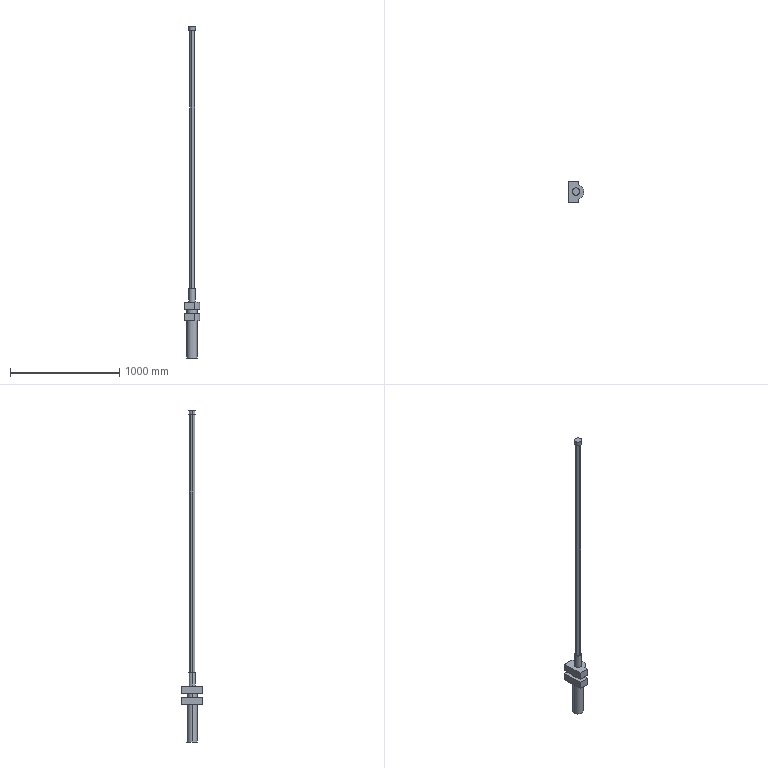Part | SolidWorks | features ICE 4, Extrusion 1, Revolution 1 | 1 solid | 34 faces | box 145 x 200 x 3045 mm | volume 9881039 mm3 | plane 24 | cylinder 8 | cone 2 | commonest cylinder face diameters 92.4 x4 60 x2 145 x2
STEP:
#1=CARTESIAN_POINT('',(46.2,0.,340.));
#2=VERTEX_POINT('',#1);
#3=CARTESIAN_POINT('',(-46.2,0.,340.));
#4=VERTEX_POINT('',#3);
#5=CARTESIAN_POINT('',(0.,0.,340.));
#6=DIRECTION('',(0.,0.,1.));
#7=DIRECTION('',(1.,0.,0.));
#8=AXIS2_PLACEMENT_3D('',#5,#6,#7);
#9=CIRCLE('',#8,46.2);
#10=EDGE_CURVE('',#2,#4,#9,.T.);
#11=ORIENTED_EDGE('',*,*,#10,.F.);
#12=CARTESIAN_POINT('',(46.2,0.,0.));
#13=VERTEX_POINT('',#12);
#14=CARTESIAN_POINT('',(46.2,0.,445.));
#15=DIRECTION('',(0.,0.,-1.));
#16=VECTOR('',#15,1000.);
#17=LINE('',#14,#16);
#18=EDGE_CURVE('',#2,#13,#17,.T.);
#19=ORIENTED_EDGE('',*,*,#18,.T.);
#20=CARTESIAN_POINT('',(-46.2,0.,0.));
#21=VERTEX_POINT('',#20);
#22=CARTESIAN_POINT('',(0.,0.,0.));
#23=DIRECTION('',(0.,0.,1.));
#24=DIRECTION('',(1.,0.,0.));
#25=AXIS2_PLACEMENT_3D('',#22,#23,#24);
#26=CIRCLE('',#25,46.2);
#27=EDGE_CURVE('',#13,#21,#26,.T.);
#28=ORIENTED_EDGE('',*,*,#27,.T.);
#29=CARTESIAN_POINT('',(-46.2,0.,445.));
#30=DIRECTION('',(0.,0.,-1.));
#31=VECTOR('',#30,1000.);
#32=LINE('',#29,#31);
#33=EDGE_CURVE('',#4,#21,#32,.T.);
#34=ORIENTED_EDGE('',*,*,#33,.F.);
#35=EDGE_LOOP('',(#11,#19,#28,#34));
#36=FACE_OUTER_BOUND('',#35,.T.);
#37=CARTESIAN_POINT('',(0.,0.,445.));
#38=DIRECTION('',(0.,0.,-1.));
#39=DIRECTION('',(-1.,0.,0.));
#40=AXIS2_PLACEMENT_3D('',#37,#38,#39);
#41=CYLINDRICAL_SURFACE('',#40,46.2);
#42=ADVANCED_FACE('',(#36),#41,.T.);
#43=CARTESIAN_POINT('',(46.2,0.,445.));
#44=VERTEX_POINT('',#43);
#45=CARTESIAN_POINT('',(-46.2,0.,445.));
#46=VERTEX_POINT('',#45);
#47=CARTESIAN_POINT('',(0.,0.,445.));
#48=DIRECTION('',(0.,0.,1.));
#49=DIRECTION('',(1.,0.,0.));
#50=AXIS2_PLACEMENT_3D('',#47,#48,#49);
#51=CIRCLE('',#50,46.2);
#52=EDGE_CURVE('',#44,#46,#51,.T.);
#53=ORIENTED_EDGE('',*,*,#52,.F.);
#54=CARTESIAN_POINT('',(46.2,0.,408.));
#55=VERTEX_POINT('',#54);
#56=CARTESIAN_POINT('',(46.2,0.,445.));
#57=DIRECTION('',(0.,0.,-1.));
#58=VECTOR('',#57,1000.);
#59=LINE('',#56,#58);
#60=EDGE_CURVE('',#44,#55,#59,.T.);
#61=ORIENTED_EDGE('',*,*,#60,.T.);
#62=CARTESIAN_POINT('',(-46.2,0.,408.));
#63=VERTEX_POINT('',#62);
#64=CARTESIAN_POINT('',(0.,0.,408.));
#65=DIRECTION('',(0.,0.,1.));
#66=DIRECTION('',(1.,0.,0.));
#67=AXIS2_PLACEMENT_3D('',#64,#65,#66);
#68=CIRCLE('',#67,46.2);
#69=EDGE_CURVE('',#55,#63,#68,.T.);
#70=ORIENTED_EDGE('',*,*,#69,.T.);
#71=CARTESIAN_POINT('',(-46.2,0.,445.));
#72=DIRECTION('',(0.,0.,-1.));
#73=VECTOR('',#72,1000.);
#74=LINE('',#71,#73);
#75=EDGE_CURVE('',#46,#63,#74,.T.);
#76=ORIENTED_EDGE('',*,*,#75,.F.);
#77=EDGE_LOOP('',(#53,#61,#70,#76));
#78=FACE_OUTER_BOUND('',#77,.T.);
#79=CARTESIAN_POINT('',(0.,0.,445.));
#80=DIRECTION('',(0.,0.,-1.));
#81=DIRECTION('',(-1.,0.,0.));
#82=AXIS2_PLACEMENT_3D('',#79,#80,#81);
#83=CYLINDRICAL_SURFACE('',#82,46.2);
#84=ADVANCED_FACE('',(#78),#83,.T.);
#85=CARTESIAN_POINT('',(-29.4,0.,3000.));
#86=VERTEX_POINT('',#85);
#87=CARTESIAN_POINT('',(29.4,0.,3000.));
#88=VERTEX_POINT('',#87);
#89=CARTESIAN_POINT('',(0.,0.,3000.));
#90=DIRECTION('',(0.,0.,-1.));
#91=DIRECTION('',(-1.,0.,0.));
#92=AXIS2_PLACEMENT_3D('',#89,#90,#91);
#93=CIRCLE('',#92,29.4);
#94=EDGE_CURVE('',#86,#88,#93,.T.);
#95=ORIENTED_EDGE('',*,*,#94,.F.);
#96=CARTESIAN_POINT('',(-33.3,0.,3045.));
#97=VERTEX_POINT('',#96);
#98=CARTESIAN_POINT('',(-33.3,0.,3045.));
#99=DIRECTION('',(-0.08634,0.,0.9963));
#100=VECTOR('',#99,1000.);
#101=LINE('',#98,#100);
#102=EDGE_CURVE('',#86,#97,#101,.T.);
#103=ORIENTED_EDGE('',*,*,#102,.T.);
#104=CARTESIAN_POINT('',(33.3,0.,3045.));
#105=VERTEX_POINT('',#104);
#106=CARTESIAN_POINT('',(0.,0.,3045.));
#107=DIRECTION('',(0.,0.,-1.));
#108=DIRECTION('',(-1.,0.,0.));
#109=AXIS2_PLACEMENT_3D('',#106,#107,#108);
#110=CIRCLE('',#109,33.3);
#111=EDGE_CURVE('',#97,#105,#110,.T.);
#112=ORIENTED_EDGE('',*,*,#111,.T.);
#113=CARTESIAN_POINT('',(33.3,0.,3045.));
#114=DIRECTION('',(0.08634,0.,0.9963));
#115=VECTOR('',#114,1000.);
#116=LINE('',#113,#115);
#117=EDGE_CURVE('',#88,#105,#116,.T.);
#118=ORIENTED_EDGE('',*,*,#117,.F.);
#119=EDGE_LOOP('',(#95,#103,#112,#118));
#120=FACE_OUTER_BOUND('',#119,.T.);
#121=CARTESIAN_POINT('',(0.,0.,3045.));
#122=DIRECTION('',(0.,0.,1.));
#123=DIRECTION('',(1.,0.,0.));
#124=AXIS2_PLACEMENT_3D('',#121,#122,#123);
#125=CONICAL_SURFACE('',#124,33.3,0.08645);
#126=ADVANCED_FACE('',(#120),#125,.T.);
#127=CARTESIAN_POINT('',(30.,0.,640.));
#128=VERTEX_POINT('',#127);
#129=CARTESIAN_POINT('',(-30.,0.,640.));
#130=VERTEX_POINT('',#129);
#131=CARTESIAN_POINT('',(0.,0.,640.));
#132=DIRECTION('',(0.,0.,1.));
#133=DIRECTION('',(1.,0.,0.));
#134=AXIS2_PLACEMENT_3D('',#131,#132,#133);
#135=CIRCLE('',#134,30.);
#136=EDGE_CURVE('',#128,#130,#135,.T.);
#137=ORIENTED_EDGE('',*,*,#136,.F.);
#138=CARTESIAN_POINT('',(30.,0.,513.));
#139=VERTEX_POINT('',#138);
#140=CARTESIAN_POINT('',(30.,0.,640.));
#141=DIRECTION('',(0.,0.,-1.));
#142=VECTOR('',#141,1000.);
#143=LINE('',#140,#142);
#144=EDGE_CURVE('',#128,#139,#143,.T.);
#145=ORIENTED_EDGE('',*,*,#144,.T.);
#146=CARTESIAN_POINT('',(-30.,0.,513.));
#147=VERTEX_POINT('',#146);
#148=CARTESIAN_POINT('',(0.,0.,513.));
#149=DIRECTION('',(0.,0.,1.));
#150=DIRECTION('',(1.,0.,0.));
#151=AXIS2_PLACEMENT_3D('',#148,#149,#150);
#152=CIRCLE('',#151,30.);
#153=EDGE_CURVE('',#139,#147,#152,.T.);
#154=ORIENTED_EDGE('',*,*,#153,.T.);
#155=CARTESIAN_POINT('',(-30.,0.,640.));
#156=DIRECTION('',(0.,0.,-1.));
#157=VECTOR('',#156,1000.);
#158=LINE('',#155,#157);
#159=EDGE_CURVE('',#130,#147,#158,.T.);
#160=ORIENTED_EDGE('',*,*,#159,.F.);
#161=EDGE_LOOP('',(#137,#145,#154,#160));
#162=FACE_OUTER_BOUND('',#161,.T.);
#163=CARTESIAN_POINT('',(0.,0.,640.));
#164=DIRECTION('',(0.,0.,-1.));
#165=DIRECTION('',(-1.,0.,0.));
#166=AXIS2_PLACEMENT_3D('',#163,#164,#165);
#167=CYLINDRICAL_SURFACE('',#166,30.);
#168=ADVANCED_FACE('',(#162),#167,.T.);
#169=CARTESIAN_POINT('',(0.,0.,640.));
#170=DIRECTION('',(0.,0.,1.));
#171=DIRECTION('',(1.,0.,0.));
#172=AXIS2_PLACEMENT_3D('',#169,#170,#171);
#173=CIRCLE('',#172,30.);
#174=EDGE_CURVE('',#130,#128,#173,.T.);
#175=ORIENTED_EDGE('',*,*,#174,.T.);
#176=ORIENTED_EDGE('',*,*,#136,.T.);
#177=EDGE_LOOP('',(#175,#176));
#178=FACE_OUTER_BOUND('',#177,.T.);
#179=CARTESIAN_POINT('',(18.342,-15.861,640.));
#180=VERTEX_POINT('',#179);
#181=CARTESIAN_POINT('',(22.907,7.954,640.));
#182=VERTEX_POINT('',#181);
#183=CARTESIAN_POINT('',(18.342,-15.861,640.));
#184=DIRECTION('',(0.1883,0.9821,0.));
#185=VECTOR('',#184,1000.);
#186=LINE('',#183,#185);
#187=EDGE_CURVE('',#180,#182,#186,.T.);
#188=ORIENTED_EDGE('',*,*,#187,.F.);
#189=CARTESIAN_POINT('',(-4.565,-23.815,640.));
#190=VERTEX_POINT('',#189);
#191=CARTESIAN_POINT('',(-4.565,-23.815,640.));
#192=DIRECTION('',(0.9447,0.328,0.));
#193=VECTOR('',#192,1000.);
#194=LINE('',#191,#193);
#195=EDGE_CURVE('',#190,#180,#194,.T.);
#196=ORIENTED_EDGE('',*,*,#195,.F.);
#197=CARTESIAN_POINT('',(-22.907,-7.954,640.));
#198=VERTEX_POINT('',#197);
#199=CARTESIAN_POINT('',(-22.907,-7.954,640.));
#200=DIRECTION('',(0.7564,-0.6541,0.));
#201=VECTOR('',#200,1000.);
#202=LINE('',#199,#201);
#203=EDGE_CURVE('',#198,#190,#202,.T.);
#204=ORIENTED_EDGE('',*,*,#203,.F.);
#205=CARTESIAN_POINT('',(-18.342,15.861,640.));
#206=VERTEX_POINT('',#205);
#207=CARTESIAN_POINT('',(-18.342,15.861,640.));
#208=DIRECTION('',(-0.1883,-0.9821,0.));
#209=VECTOR('',#208,1000.);
#210=LINE('',#207,#209);
#211=EDGE_CURVE('',#206,#198,#210,.T.);
#212=ORIENTED_EDGE('',*,*,#211,.F.);
#213=CARTESIAN_POINT('',(4.565,23.815,640.));
#214=VERTEX_POINT('',#213);
#215=CARTESIAN_POINT('',(4.565,23.815,640.));
#216=DIRECTION('',(-0.9447,-0.328,0.));
#217=VECTOR('',#216,1000.);
#218=LINE('',#215,#217);
#219=EDGE_CURVE('',#214,#206,#218,.T.);
#220=ORIENTED_EDGE('',*,*,#219,.F.);
#221=CARTESIAN_POINT('',(22.907,7.954,640.));
#222=DIRECTION('',(-0.7564,0.6541,0.));
#223=VECTOR('',#222,1000.);
#224=LINE('',#221,#223);
#225=EDGE_CURVE('',#182,#214,#224,.T.);
#226=ORIENTED_EDGE('',*,*,#225,.F.);
#227=EDGE_LOOP('',(#188,#196,#204,#212,#220,#226));
#228=FACE_BOUND('',#227,.T.);
#229=CARTESIAN_POINT('',(0.,0.,640.));
#230=DIRECTION('',(0.,0.,1.));
#231=DIRECTION('',(1.,0.,0.));
#232=AXIS2_PLACEMENT_3D('',#229,#230,#231);
#233=PLANE('',#232);
#234=ADVANCED_FACE('',(#178,#228),#233,.T.);
#235=ORIENTED_EDGE('',*,*,#144,.F.);
#236=ORIENTED_EDGE('',*,*,#174,.F.);
#237=ORIENTED_EDGE('',*,*,#159,.T.);
#238=CARTESIAN_POINT('',(0.,0.,513.));
#239=DIRECTION('',(0.,0.,1.));
#240=DIRECTION('',(1.,0.,0.));
#241=AXIS2_PLACEMENT_3D('',#238,#239,#240);
#242=CIRCLE('',#241,30.);
#243=EDGE_CURVE('',#147,#139,#242,.T.);
#244=ORIENTED_EDGE('',*,*,#243,.T.);
#245=EDGE_LOOP('',(#235,#236,#237,#244));
#246=FACE_OUTER_BOUND('',#245,.T.);
#247=CARTESIAN_POINT('',(0.,0.,640.));
#248=DIRECTION('',(0.,0.,-1.));
#249=DIRECTION('',(-1.,0.,0.));
#250=AXIS2_PLACEMENT_3D('',#247,#248,#249);
#251=CYLINDRICAL_SURFACE('',#250,30.);
#252=ADVANCED_FACE('',(#246),#251,.T.);
#253=ORIENTED_EDGE('',*,*,#195,.T.);
#254=CARTESIAN_POINT('',(18.342,-15.861,3000.));
#255=VERTEX_POINT('',#254);
#256=CARTESIAN_POINT('',(18.342,-15.861,3000.));
#257=DIRECTION('',(0.,0.,-1.));
#258=VECTOR('',#257,1000.);
#259=LINE('',#256,#258);
#260=EDGE_CURVE('',#255,#180,#259,.T.);
#261=ORIENTED_EDGE('',*,*,#260,.F.);
#262=CARTESIAN_POINT('',(-4.565,-23.815,3000.));
#263=VERTEX_POINT('',#262);
#264=CARTESIAN_POINT('',(-4.565,-23.815,3000.));
#265=DIRECTION('',(0.9447,0.328,0.));
#266=VECTOR('',#265,1000.);
#267=LINE('',#264,#266);
#268=EDGE_CURVE('',#263,#255,#267,.T.);
#269=ORIENTED_EDGE('',*,*,#268,.F.);
#270=CARTESIAN_POINT('',(-4.565,-23.815,3000.));
#271=DIRECTION('',(0.,0.,-1.));
#272=VECTOR('',#271,1000.);
#273=LINE('',#270,#272);
#274=EDGE_CURVE('',#263,#190,#273,.T.);
#275=ORIENTED_EDGE('',*,*,#274,.T.);
#276=EDGE_LOOP('',(#253,#261,#269,#275));
#277=FACE_OUTER_BOUND('',#276,.T.);
#278=CARTESIAN_POINT('',(-4.565,-23.815,3000.));
#279=DIRECTION('',(-0.328,0.9447,0.));
#280=DIRECTION('',(-0.9447,-0.328,0.));
#281=AXIS2_PLACEMENT_3D('',#278,#279,#280);
#282=PLANE('',#281);
#283=ADVANCED_FACE('',(#277),#282,.F.);
#284=ORIENTED_EDGE('',*,*,#187,.T.);
#285=CARTESIAN_POINT('',(22.907,7.954,3000.));
#286=VERTEX_POINT('',#285);
#287=CARTESIAN_POINT('',(22.907,7.954,3000.));
#288=DIRECTION('',(0.,0.,-1.));
#289=VECTOR('',#288,1000.);
#290=LINE('',#287,#289);
#291=EDGE_CURVE('',#286,#182,#290,.T.);
#292=ORIENTED_EDGE('',*,*,#291,.F.);
#293=CARTESIAN_POINT('',(18.342,-15.861,3000.));
#294=DIRECTION('',(0.1883,0.9821,0.));
#295=VECTOR('',#294,1000.);
#296=LINE('',#293,#295);
#297=EDGE_CURVE('',#255,#286,#296,.T.);
#298=ORIENTED_EDGE('',*,*,#297,.F.);
#299=ORIENTED_EDGE('',*,*,#260,.T.);
#300=EDGE_LOOP('',(#284,#292,#298,#299));
#301=FACE_OUTER_BOUND('',#300,.T.);
#302=CARTESIAN_POINT('',(18.342,-15.861,3000.));
#303=DIRECTION('',(-0.9821,0.1883,0.));
#304=DIRECTION('',(-0.1883,-0.9821,0.));
#305=AXIS2_PLACEMENT_3D('',#302,#303,#304);
#306=PLANE('',#305);
#307=ADVANCED_FACE('',(#301),#306,.F.);
#308=ORIENTED_EDGE('',*,*,#225,.T.);
#309=CARTESIAN_POINT('',(4.565,23.815,3000.));
#310=VERTEX_POINT('',#309);
#311=CARTESIAN_POINT('',(4.565,23.815,3000.));
#312=DIRECTION('',(0.,0.,-1.));
#313=VECTOR('',#312,1000.);
#314=LINE('',#311,#313);
#315=EDGE_CURVE('',#310,#214,#314,.T.);
#316=ORIENTED_EDGE('',*,*,#315,.F.);
#317=CARTESIAN_POINT('',(22.907,7.954,3000.));
#318=DIRECTION('',(-0.7564,0.6541,0.));
#319=VECTOR('',#318,1000.);
#320=LINE('',#317,#319);
#321=EDGE_CURVE('',#286,#310,#320,.T.);
#322=ORIENTED_EDGE('',*,*,#321,.F.);
#323=ORIENTED_EDGE('',*,*,#291,.T.);
#324=EDGE_LOOP('',(#308,#316,#322,#323));
#325=FACE_OUTER_BOUND('',#324,.T.);
#326=CARTESIAN_POINT('',(22.907,7.954,3000.));
#327=DIRECTION('',(-0.6541,-0.7564,0.));
#328=DIRECTION('',(0.7564,-0.6541,0.));
#329=AXIS2_PLACEMENT_3D('',#326,#327,#328);
#330=PLANE('',#329);
#331=ADVANCED_FACE('',(#325),#330,.F.);
#332=ORIENTED_EDGE('',*,*,#219,.T.);
#333=CARTESIAN_POINT('',(-18.342,15.861,3000.));
#334=VERTEX_POINT('',#333);
#335=CARTESIAN_POINT('',(-18.342,15.861,3000.));
#336=DIRECTION('',(0.,0.,-1.));
#337=VECTOR('',#336,1000.);
#338=LINE('',#335,#337);
#339=EDGE_CURVE('',#334,#206,#338,.T.);
#340=ORIENTED_EDGE('',*,*,#339,.F.);
#341=CARTESIAN_POINT('',(4.565,23.815,3000.));
#342=DIRECTION('',(-0.9447,-0.328,0.));
#343=VECTOR('',#342,1000.);
#344=LINE('',#341,#343);
#345=EDGE_CURVE('',#310,#334,#344,.T.);
#346=ORIENTED_EDGE('',*,*,#345,.F.);
#347=ORIENTED_EDGE('',*,*,#315,.T.);
#348=EDGE_LOOP('',(#332,#340,#346,#347));
#349=FACE_OUTER_BOUND('',#348,.T.);
#350=CARTESIAN_POINT('',(4.565,23.815,3000.));
#351=DIRECTION('',(0.328,-0.9447,0.));
#352=DIRECTION('',(0.9447,0.328,0.));
#353=AXIS2_PLACEMENT_3D('',#350,#351,#352);
#354=PLANE('',#353);
#355=ADVANCED_FACE('',(#349),#354,.F.);
#356=ORIENTED_EDGE('',*,*,#211,.T.);
#357=CARTESIAN_POINT('',(-22.907,-7.954,3000.));
#358=VERTEX_POINT('',#357);
#359=CARTESIAN_POINT('',(-22.907,-7.954,3000.));
#360=DIRECTION('',(0.,0.,-1.));
#361=VECTOR('',#360,1000.);
#362=LINE('',#359,#361);
#363=EDGE_CURVE('',#358,#198,#362,.T.);
#364=ORIENTED_EDGE('',*,*,#363,.F.);
#365=CARTESIAN_POINT('',(-18.342,15.861,3000.));
#366=DIRECTION('',(-0.1883,-0.9821,0.));
#367=VECTOR('',#366,1000.);
#368=LINE('',#365,#367);
#369=EDGE_CURVE('',#334,#358,#368,.T.);
#370=ORIENTED_EDGE('',*,*,#369,.F.);
#371=ORIENTED_EDGE('',*,*,#339,.T.);
#372=EDGE_LOOP('',(#356,#364,#370,#371));
#373=FACE_OUTER_BOUND('',#372,.T.);
#374=CARTESIAN_POINT('',(-18.342,15.861,3000.));
#375=DIRECTION('',(0.9821,-0.1883,0.));
#376=DIRECTION('',(0.1883,0.9821,0.));
#377=AXIS2_PLACEMENT_3D('',#374,#375,#376);
#378=PLANE('',#377);
#379=ADVANCED_FACE('',(#373),#378,.F.);
#380=ORIENTED_EDGE('',*,*,#203,.T.);
#381=ORIENTED_EDGE('',*,*,#274,.F.);
#382=CARTESIAN_POINT('',(-22.907,-7.954,3000.));
#383=DIRECTION('',(0.7564,-0.6541,0.));
#384=VECTOR('',#383,1000.);
#385=LINE('',#382,#384);
#386=EDGE_CURVE('',#358,#263,#385,.T.);
#387=ORIENTED_EDGE('',*,*,#386,.F.);
#388=ORIENTED_EDGE('',*,*,#363,.T.);
#389=EDGE_LOOP('',(#380,#381,#387,#388));
#390=FACE_OUTER_BOUND('',#389,.T.);
#391=CARTESIAN_POINT('',(-22.907,-7.954,3000.));
#392=DIRECTION('',(0.6541,0.7564,0.));
#393=DIRECTION('',(-0.7564,0.6541,0.));
#394=AXIS2_PLACEMENT_3D('',#391,#392,#393);
#395=PLANE('',#394);
#396=ADVANCED_FACE('',(#390),#395,.F.);
#397=CARTESIAN_POINT('',(0.,0.,3000.));
#398=DIRECTION('',(0.,0.,-1.));
#399=DIRECTION('',(-1.,0.,0.));
#400=AXIS2_PLACEMENT_3D('',#397,#398,#399);
#401=CIRCLE('',#400,29.4);
#402=EDGE_CURVE('',#88,#86,#401,.T.);
#403=ORIENTED_EDGE('',*,*,#402,.T.);
#404=ORIENTED_EDGE('',*,*,#94,.T.);
#405=EDGE_LOOP('',(#403,#404));
#406=FACE_OUTER_BOUND('',#405,.T.);
#407=ORIENTED_EDGE('',*,*,#386,.T.);
#408=ORIENTED_EDGE('',*,*,#268,.T.);
#409=ORIENTED_EDGE('',*,*,#297,.T.);
#410=ORIENTED_EDGE('',*,*,#321,.T.);
#411=ORIENTED_EDGE('',*,*,#345,.T.);
#412=ORIENTED_EDGE('',*,*,#369,.T.);
#413=EDGE_LOOP('',(#407,#408,#409,#410,#411,#412));
#414=FACE_BOUND('',#413,.T.);
#415=CARTESIAN_POINT('',(29.4,0.,3000.));
#416=DIRECTION('',(0.,0.,1.));
#417=DIRECTION('',(1.,0.,0.));
#418=AXIS2_PLACEMENT_3D('',#415,#416,#417);
#419=PLANE('',#418);
#420=ADVANCED_FACE('',(#406,#414),#419,.F.);
#421=ORIENTED_EDGE('',*,*,#102,.F.);
#422=ORIENTED_EDGE('',*,*,#402,.F.);
#423=ORIENTED_EDGE('',*,*,#117,.T.);
#424=CARTESIAN_POINT('',(0.,0.,3045.));
#425=DIRECTION('',(0.,0.,-1.));
#426=DIRECTION('',(-1.,0.,0.));
#427=AXIS2_PLACEMENT_3D('',#424,#425,#426);
#428=CIRCLE('',#427,33.3);
#429=EDGE_CURVE('',#105,#97,#428,.T.);
#430=ORIENTED_EDGE('',*,*,#429,.T.);
#431=EDGE_LOOP('',(#421,#422,#423,#430));
#432=FACE_OUTER_BOUND('',#431,.T.);
#433=CARTESIAN_POINT('',(0.,0.,3045.));
#434=DIRECTION('',(0.,0.,1.));
#435=DIRECTION('',(1.,0.,0.));
#436=AXIS2_PLACEMENT_3D('',#433,#434,#435);
#437=CONICAL_SURFACE('',#436,33.3,0.08645);
#438=ADVANCED_FACE('',(#432),#437,.T.);
#439=ORIENTED_EDGE('',*,*,#429,.F.);
#440=ORIENTED_EDGE('',*,*,#111,.F.);
#441=EDGE_LOOP('',(#439,#440));
#442=FACE_OUTER_BOUND('',#441,.T.);
#443=CARTESIAN_POINT('',(33.3,0.,3045.));
#444=DIRECTION('',(0.,0.,-1.));
#445=DIRECTION('',(-1.,0.,0.));
#446=AXIS2_PLACEMENT_3D('',#443,#444,#445);
#447=PLANE('',#446);
#448=ADVANCED_FACE('',(#442),#447,.F.);
#449=CARTESIAN_POINT('',(20.,100.,513.));
#450=VERTEX_POINT('',#449);
#451=CARTESIAN_POINT('',(-72.5,100.,513.));
#452=VERTEX_POINT('',#451);
#453=CARTESIAN_POINT('',(0.,100.,513.));
#454=DIRECTION('',(-1.,0.,0.));
#455=VECTOR('',#454,1000.);
#456=LINE('',#453,#455);
#457=EDGE_CURVE('',#450,#452,#456,.T.);
#458=ORIENTED_EDGE('',*,*,#457,.T.);
#459=CARTESIAN_POINT('',(-72.5,-100.,513.));
#460=VERTEX_POINT('',#459);
#461=CARTESIAN_POINT('',(-72.5,100.,513.));
#462=DIRECTION('',(0.,-1.,0.));
#463=VECTOR('',#462,1000.);
#464=LINE('',#461,#463);
#465=EDGE_CURVE('',#452,#460,#464,.T.);
#466=ORIENTED_EDGE('',*,*,#465,.T.);
#467=CARTESIAN_POINT('',(20.,-100.,513.));
#468=VERTEX_POINT('',#467);
#469=CARTESIAN_POINT('',(0.,-100.,513.));
#470=DIRECTION('',(1.,0.,0.));
#471=VECTOR('',#470,1000.);
#472=LINE('',#469,#471);
#473=EDGE_CURVE('',#460,#468,#472,.T.);
#474=ORIENTED_EDGE('',*,*,#473,.T.);
#475=CARTESIAN_POINT('',(20.,-69.687,513.));
#476=VERTEX_POINT('',#475);
#477=CARTESIAN_POINT('',(20.,-100.,513.));
#478=DIRECTION('',(0.,1.,0.));
#479=VECTOR('',#478,1000.);
#480=LINE('',#477,#479);
#481=EDGE_CURVE('',#468,#476,#480,.T.);
#482=ORIENTED_EDGE('',*,*,#481,.T.);
#483=CARTESIAN_POINT('',(20.,69.687,513.));
#484=VERTEX_POINT('',#483);
#485=CARTESIAN_POINT('',(0.,0.,513.));
#486=DIRECTION('',(0.,0.,1.));
#487=DIRECTION('',(1.,0.,0.));
#488=AXIS2_PLACEMENT_3D('',#485,#486,#487);
#489=CIRCLE('',#488,72.5);
#490=EDGE_CURVE('',#476,#484,#489,.T.);
#491=ORIENTED_EDGE('',*,*,#490,.T.);
#492=CARTESIAN_POINT('',(20.,100.,513.));
#493=DIRECTION('',(0.,1.,0.));
#494=VECTOR('',#493,1000.);
#495=LINE('',#492,#494);
#496=EDGE_CURVE('',#484,#450,#495,.T.);
#497=ORIENTED_EDGE('',*,*,#496,.T.);
#498=EDGE_LOOP('',(#458,#466,#474,#482,#491,#497));
#499=FACE_OUTER_BOUND('',#498,.T.);
#500=ORIENTED_EDGE('',*,*,#243,.F.);
#501=ORIENTED_EDGE('',*,*,#153,.F.);
#502=EDGE_LOOP('',(#500,#501));
#503=FACE_BOUND('',#502,.T.);
#504=CARTESIAN_POINT('',(0.,0.,513.));
#505=DIRECTION('',(0.,0.,1.));
#506=DIRECTION('',(1.,0.,0.));
#507=AXIS2_PLACEMENT_3D('',#504,#505,#506);
#508=PLANE('',#507);
#509=ADVANCED_FACE('',(#499,#503),#508,.T.);
#510=CARTESIAN_POINT('',(20.,100.,445.));
#511=VERTEX_POINT('',#510);
#512=CARTESIAN_POINT('',(-72.5,100.,445.));
#513=VERTEX_POINT('',#512);
#514=CARTESIAN_POINT('',(0.,100.,445.));
#515=DIRECTION('',(-1.,0.,0.));
#516=VECTOR('',#515,1000.);
#517=LINE('',#514,#516);
#518=EDGE_CURVE('',#511,#513,#517,.T.);
#519=ORIENTED_EDGE('',*,*,#518,.F.);
#520=CARTESIAN_POINT('',(20.,69.687,445.));
#521=VERTEX_POINT('',#520);
#522=CARTESIAN_POINT('',(20.,100.,445.));
#523=DIRECTION('',(0.,1.,0.));
#524=VECTOR('',#523,1000.);
#525=LINE('',#522,#524);
#526=EDGE_CURVE('',#521,#511,#525,.T.);
#527=ORIENTED_EDGE('',*,*,#526,.F.);
#528=CARTESIAN_POINT('',(20.,-69.687,445.));
#529=VERTEX_POINT('',#528);
#530=CARTESIAN_POINT('',(0.,0.,445.));
#531=DIRECTION('',(0.,0.,1.));
#532=DIRECTION('',(1.,0.,0.));
#533=AXIS2_PLACEMENT_3D('',#530,#531,#532);
#534=CIRCLE('',#533,72.5);
#535=EDGE_CURVE('',#529,#521,#534,.T.);
#536=ORIENTED_EDGE('',*,*,#535,.F.);
#537=CARTESIAN_POINT('',(20.,-100.,445.));
#538=VERTEX_POINT('',#537);
#539=CARTESIAN_POINT('',(20.,-100.,445.));
#540=DIRECTION('',(0.,1.,0.));
#541=VECTOR('',#540,1000.);
#542=LINE('',#539,#541);
#543=EDGE_CURVE('',#538,#529,#542,.T.);
#544=ORIENTED_EDGE('',*,*,#543,.F.);
#545=CARTESIAN_POINT('',(-72.5,-100.,445.));
#546=VERTEX_POINT('',#545);
#547=CARTESIAN_POINT('',(0.,-100.,445.));
#548=DIRECTION('',(1.,0.,0.));
#549=VECTOR('',#548,1000.);
#550=LINE('',#547,#549);
#551=EDGE_CURVE('',#546,#538,#550,.T.);
#552=ORIENTED_EDGE('',*,*,#551,.F.);
#553=CARTESIAN_POINT('',(-72.5,100.,445.));
#554=DIRECTION('',(0.,-1.,0.));
#555=VECTOR('',#554,1000.);
#556=LINE('',#553,#555);
#557=EDGE_CURVE('',#513,#546,#556,.T.);
#558=ORIENTED_EDGE('',*,*,#557,.F.);
#559=EDGE_LOOP('',(#519,#527,#536,#544,#552,#558));
#560=FACE_OUTER_BOUND('',#559,.T.);
#561=CARTESIAN_POINT('',(0.,0.,445.));
#562=DIRECTION('',(0.,0.,1.));
#563=DIRECTION('',(1.,0.,0.));
#564=AXIS2_PLACEMENT_3D('',#561,#562,#563);
#565=CIRCLE('',#564,46.2);
#566=EDGE_CURVE('',#46,#44,#565,.T.);
#567=ORIENTED_EDGE('',*,*,#566,.T.);
#568=ORIENTED_EDGE('',*,*,#52,.T.);
#569=EDGE_LOOP('',(#567,#568));
#570=FACE_BOUND('',#569,.T.);
#571=CARTESIAN_POINT('',(0.,0.,445.));
#572=DIRECTION('',(0.,0.,1.));
#573=DIRECTION('',(1.,0.,0.));
#574=AXIS2_PLACEMENT_3D('',#571,#572,#573);
#575=PLANE('',#574);
#576=ADVANCED_FACE('',(#560,#570),#575,.F.);
#577=ORIENTED_EDGE('',*,*,#518,.T.);
#578=CARTESIAN_POINT('',(-72.5,100.,513.));
#579=DIRECTION('',(0.,0.,-1.));
#580=VECTOR('',#579,1000.);
#581=LINE('',#578,#580);
#582=EDGE_CURVE('',#452,#513,#581,.T.);
#583=ORIENTED_EDGE('',*,*,#582,.F.);
#584=ORIENTED_EDGE('',*,*,#457,.F.);
#585=CARTESIAN_POINT('',(20.,100.,513.));
#586=DIRECTION('',(0.,0.,-1.));
#587=VECTOR('',#586,1000.);
#588=LINE('',#585,#587);
#589=EDGE_CURVE('',#450,#511,#588,.T.);
#590=ORIENTED_EDGE('',*,*,#589,.T.);
#591=EDGE_LOOP('',(#577,#583,#584,#590));
#592=FACE_OUTER_BOUND('',#591,.T.);
#593=CARTESIAN_POINT('',(0.,100.,513.));
#594=DIRECTION('',(0.,-1.,0.));
#595=DIRECTION('',(1.,0.,0.));
#596=AXIS2_PLACEMENT_3D('',#593,#594,#595);
#597=PLANE('',#596);
#598=ADVANCED_FACE('',(#592),#597,.F.);
#599=ORIENTED_EDGE('',*,*,#557,.T.);
#600=CARTESIAN_POINT('',(-72.5,-100.,513.));
#601=DIRECTION('',(0.,0.,-1.));
#602=VECTOR('',#601,1000.);
#603=LINE('',#600,#602);
#604=EDGE_CURVE('',#460,#546,#603,.T.);
#605=ORIENTED_EDGE('',*,*,#604,.F.);
#606=ORIENTED_EDGE('',*,*,#465,.F.);
#607=ORIENTED_EDGE('',*,*,#582,.T.);
#608=EDGE_LOOP('',(#599,#605,#606,#607));
#609=FACE_OUTER_BOUND('',#608,.T.);
#610=CARTESIAN_POINT('',(-72.5,100.,513.));
#611=DIRECTION('',(1.,0.,0.));
#612=DIRECTION('',(0.,1.,0.));
#613=AXIS2_PLACEMENT_3D('',#610,#611,#612);
#614=PLANE('',#613);
#615=ADVANCED_FACE('',(#609),#614,.F.);
#616=ORIENTED_EDGE('',*,*,#551,.T.);
#617=CARTESIAN_POINT('',(20.,-100.,513.));
#618=DIRECTION('',(0.,0.,-1.));
#619=VECTOR('',#618,1000.);
#620=LINE('',#617,#619);
#621=EDGE_CURVE('',#468,#538,#620,.T.);
#622=ORIENTED_EDGE('',*,*,#621,.F.);
#623=ORIENTED_EDGE('',*,*,#473,.F.);
#624=ORIENTED_EDGE('',*,*,#604,.T.);
#625=EDGE_LOOP('',(#616,#622,#623,#624));
#626=FACE_OUTER_BOUND('',#625,.T.);
#627=CARTESIAN_POINT('',(0.,-100.,513.));
#628=DIRECTION('',(0.,1.,0.));
#629=DIRECTION('',(0.,0.,1.));
#630=AXIS2_PLACEMENT_3D('',#627,#628,#629);
#631=PLANE('',#630);
#632=ADVANCED_FACE('',(#626),#631,.F.);
#633=ORIENTED_EDGE('',*,*,#543,.T.);
#634=CARTESIAN_POINT('',(20.,-69.687,513.));
#635=DIRECTION('',(0.,0.,-1.));
#636=VECTOR('',#635,1000.);
#637=LINE('',#634,#636);
#638=EDGE_CURVE('',#476,#529,#637,.T.);
#639=ORIENTED_EDGE('',*,*,#638,.F.);
#640=ORIENTED_EDGE('',*,*,#481,.F.);
#641=ORIENTED_EDGE('',*,*,#621,.T.);
#642=EDGE_LOOP('',(#633,#639,#640,#641));
#643=FACE_OUTER_BOUND('',#642,.T.);
#644=CARTESIAN_POINT('',(20.,-100.,513.));
#645=DIRECTION('',(-1.,0.,0.));
#646=DIRECTION('',(0.,0.,1.));
#647=AXIS2_PLACEMENT_3D('',#644,#645,#646);
#648=PLANE('',#647);
#649=ADVANCED_FACE('',(#643),#648,.F.);
#650=ORIENTED_EDGE('',*,*,#535,.T.);
#651=CARTESIAN_POINT('',(20.,69.687,513.));
#652=DIRECTION('',(0.,0.,-1.));
#653=VECTOR('',#652,1000.);
#654=LINE('',#651,#653);
#655=EDGE_CURVE('',#484,#521,#654,.T.);
#656=ORIENTED_EDGE('',*,*,#655,.F.);
#657=ORIENTED_EDGE('',*,*,#490,.F.);
#658=ORIENTED_EDGE('',*,*,#638,.T.);
#659=EDGE_LOOP('',(#650,#656,#657,#658));
#660=FACE_OUTER_BOUND('',#659,.T.);
#661=CARTESIAN_POINT('',(0.,0.,513.));
#662=DIRECTION('',(0.,0.,-1.));
#663=DIRECTION('',(-1.,0.,0.));
#664=AXIS2_PLACEMENT_3D('',#661,#662,#663);
#665=CYLINDRICAL_SURFACE('',#664,72.5);
#666=ADVANCED_FACE('',(#660),#665,.T.);
#667=ORIENTED_EDGE('',*,*,#526,.T.);
#668=ORIENTED_EDGE('',*,*,#589,.F.);
#669=ORIENTED_EDGE('',*,*,#496,.F.);
#670=ORIENTED_EDGE('',*,*,#655,.T.);
#671=EDGE_LOOP('',(#667,#668,#669,#670));
#672=FACE_OUTER_BOUND('',#671,.T.);
#673=CARTESIAN_POINT('',(20.,100.,513.));
#674=DIRECTION('',(-1.,0.,0.));
#675=DIRECTION('',(0.,-1.,0.));
#676=AXIS2_PLACEMENT_3D('',#673,#674,#675);
#677=PLANE('',#676);
#678=ADVANCED_FACE('',(#672),#677,.F.);
#679=ORIENTED_EDGE('',*,*,#60,.F.);
#680=ORIENTED_EDGE('',*,*,#566,.F.);
#681=ORIENTED_EDGE('',*,*,#75,.T.);
#682=CARTESIAN_POINT('',(0.,0.,408.));
#683=DIRECTION('',(0.,0.,1.));
#684=DIRECTION('',(1.,0.,0.));
#685=AXIS2_PLACEMENT_3D('',#682,#683,#684);
#686=CIRCLE('',#685,46.2);
#687=EDGE_CURVE('',#63,#55,#686,.T.);
#688=ORIENTED_EDGE('',*,*,#687,.T.);
#689=EDGE_LOOP('',(#679,#680,#681,#688));
#690=FACE_OUTER_BOUND('',#689,.T.);
#691=CARTESIAN_POINT('',(0.,0.,445.));
#692=DIRECTION('',(0.,0.,-1.));
#693=DIRECTION('',(-1.,0.,0.));
#694=AXIS2_PLACEMENT_3D('',#691,#692,#693);
#695=CYLINDRICAL_SURFACE('',#694,46.2);
#696=ADVANCED_FACE('',(#690),#695,.T.);
#697=CARTESIAN_POINT('',(-72.5,100.,408.));
#698=VERTEX_POINT('',#697);
#699=CARTESIAN_POINT('',(-72.5,-100.,408.));
#700=VERTEX_POINT('',#699);
#701=CARTESIAN_POINT('',(-72.5,100.,408.));
#702=DIRECTION('',(0.,-1.,0.));
#703=VECTOR('',#702,1000.);
#704=LINE('',#701,#703);
#705=EDGE_CURVE('',#698,#700,#704,.T.);
#706=ORIENTED_EDGE('',*,*,#705,.T.);
#707=CARTESIAN_POINT('',(20.,-100.,408.));
#708=VERTEX_POINT('',#707);
#709=CARTESIAN_POINT('',(-72.5,-100.,408.));
#710=DIRECTION('',(1.,0.,0.));
#711=VECTOR('',#710,1000.);
#712=LINE('',#709,#711);
#713=EDGE_CURVE('',#700,#708,#712,.T.);
#714=ORIENTED_EDGE('',*,*,#713,.T.);
#715=CARTESIAN_POINT('',(20.,-69.687,408.));
#716=VERTEX_POINT('',#715);
#717=CARTESIAN_POINT('',(20.,-100.,408.));
#718=DIRECTION('',(0.,1.,0.));
#719=VECTOR('',#718,1000.);
#720=LINE('',#717,#719);
#721=EDGE_CURVE('',#708,#716,#720,.T.);
#722=ORIENTED_EDGE('',*,*,#721,.T.);
#723=CARTESIAN_POINT('',(20.,69.687,408.));
#724=VERTEX_POINT('',#723);
#725=CARTESIAN_POINT('',(0.,0.,408.));
#726=DIRECTION('',(0.,0.,1.));
#727=DIRECTION('',(1.,0.,0.));
#728=AXIS2_PLACEMENT_3D('',#725,#726,#727);
#729=CIRCLE('',#728,72.5);
#730=EDGE_CURVE('',#716,#724,#729,.T.);
#731=ORIENTED_EDGE('',*,*,#730,.T.);
#732=CARTESIAN_POINT('',(20.,100.,408.));
#733=VERTEX_POINT('',#732);
#734=CARTESIAN_POINT('',(20.,69.687,408.));
#735=DIRECTION('',(0.,1.,0.));
#736=VECTOR('',#735,1000.);
#737=LINE('',#734,#736);
#738=EDGE_CURVE('',#724,#733,#737,.T.);
#739=ORIENTED_EDGE('',*,*,#738,.T.);
#740=CARTESIAN_POINT('',(20.,100.,408.));
#741=DIRECTION('',(-1.,0.,0.));
#742=VECTOR('',#741,1000.);
#743=LINE('',#740,#742);
#744=EDGE_CURVE('',#733,#698,#743,.T.);
#745=ORIENTED_EDGE('',*,*,#744,.T.);
#746=EDGE_LOOP('',(#706,#714,#722,#731,#739,#745));
#747=FACE_OUTER_BOUND('',#746,.T.);
#748=ORIENTED_EDGE('',*,*,#687,.F.);
#749=ORIENTED_EDGE('',*,*,#69,.F.);
#750=EDGE_LOOP('',(#748,#749));
#751=FACE_BOUND('',#750,.T.);
#752=CARTESIAN_POINT('',(0.,0.,408.));
#753=DIRECTION('',(0.,0.,1.));
#754=DIRECTION('',(1.,0.,0.));
#755=AXIS2_PLACEMENT_3D('',#752,#753,#754);
#756=PLANE('',#755);
#757=ADVANCED_FACE('',(#747,#751),#756,.T.);
#758=CARTESIAN_POINT('',(-72.5,100.,340.));
#759=VERTEX_POINT('',#758);
#760=CARTESIAN_POINT('',(-72.5,-100.,340.));
#761=VERTEX_POINT('',#760);
#762=CARTESIAN_POINT('',(-72.5,100.,340.));
#763=DIRECTION('',(0.,-1.,0.));
#764=VECTOR('',#763,1000.);
#765=LINE('',#762,#764);
#766=EDGE_CURVE('',#759,#761,#765,.T.);
#767=ORIENTED_EDGE('',*,*,#766,.F.);
#768=CARTESIAN_POINT('',(20.,100.,340.));
#769=VERTEX_POINT('',#768);
#770=CARTESIAN_POINT('',(20.,100.,340.));
#771=DIRECTION('',(-1.,0.,0.));
#772=VECTOR('',#771,1000.);
#773=LINE('',#770,#772);
#774=EDGE_CURVE('',#769,#759,#773,.T.);
#775=ORIENTED_EDGE('',*,*,#774,.F.);
#776=CARTESIAN_POINT('',(20.,69.687,340.));
#777=VERTEX_POINT('',#776);
#778=CARTESIAN_POINT('',(20.,69.687,340.));
#779=DIRECTION('',(0.,1.,0.));
#780=VECTOR('',#779,1000.);
#781=LINE('',#778,#780);
#782=EDGE_CURVE('',#777,#769,#781,.T.);
#783=ORIENTED_EDGE('',*,*,#782,.F.);
#784=CARTESIAN_POINT('',(20.,-69.687,340.));
#785=VERTEX_POINT('',#784);
#786=CARTESIAN_POINT('',(0.,0.,340.));
#787=DIRECTION('',(0.,0.,1.));
#788=DIRECTION('',(1.,0.,0.));
#789=AXIS2_PLACEMENT_3D('',#786,#787,#788);
#790=CIRCLE('',#789,72.5);
#791=EDGE_CURVE('',#785,#777,#790,.T.);
#792=ORIENTED_EDGE('',*,*,#791,.F.);
#793=CARTESIAN_POINT('',(20.,-100.,340.));
#794=VERTEX_POINT('',#793);
#795=CARTESIAN_POINT('',(20.,-100.,340.));
#796=DIRECTION('',(0.,1.,0.));
#797=VECTOR('',#796,1000.);
#798=LINE('',#795,#797);
#799=EDGE_CURVE('',#794,#785,#798,.T.);
#800=ORIENTED_EDGE('',*,*,#799,.F.);
#801=CARTESIAN_POINT('',(-72.5,-100.,340.));
#802=DIRECTION('',(1.,0.,0.));
#803=VECTOR('',#802,1000.);
#804=LINE('',#801,#803);
#805=EDGE_CURVE('',#761,#794,#804,.T.);
#806=ORIENTED_EDGE('',*,*,#805,.F.);
#807=EDGE_LOOP('',(#767,#775,#783,#792,#800,#806));
#808=FACE_OUTER_BOUND('',#807,.T.);
#809=CARTESIAN_POINT('',(0.,0.,340.));
#810=DIRECTION('',(0.,0.,1.));
#811=DIRECTION('',(1.,0.,0.));
#812=AXIS2_PLACEMENT_3D('',#809,#810,#811);
#813=CIRCLE('',#812,46.2);
#814=EDGE_CURVE('',#4,#2,#813,.T.);
#815=ORIENTED_EDGE('',*,*,#814,.T.);
#816=ORIENTED_EDGE('',*,*,#10,.T.);
#817=EDGE_LOOP('',(#815,#816));
#818=FACE_BOUND('',#817,.T.);
#819=CARTESIAN_POINT('',(0.,0.,340.));
#820=DIRECTION('',(0.,0.,1.));
#821=DIRECTION('',(1.,0.,0.));
#822=AXIS2_PLACEMENT_3D('',#819,#820,#821);
#823=PLANE('',#822);
#824=ADVANCED_FACE('',(#808,#818),#823,.F.);
#825=ORIENTED_EDGE('',*,*,#766,.T.);
#826=CARTESIAN_POINT('',(-72.5,-100.,408.));
#827=DIRECTION('',(0.,0.,-1.));
#828=VECTOR('',#827,1000.);
#829=LINE('',#826,#828);
#830=EDGE_CURVE('',#700,#761,#829,.T.);
#831=ORIENTED_EDGE('',*,*,#830,.F.);
#832=ORIENTED_EDGE('',*,*,#705,.F.);
#833=CARTESIAN_POINT('',(-72.5,100.,408.));
#834=DIRECTION('',(0.,0.,-1.));
#835=VECTOR('',#834,1000.);
#836=LINE('',#833,#835);
#837=EDGE_CURVE('',#698,#759,#836,.T.);
#838=ORIENTED_EDGE('',*,*,#837,.T.);
#839=EDGE_LOOP('',(#825,#831,#832,#838));
#840=FACE_OUTER_BOUND('',#839,.T.);
#841=CARTESIAN_POINT('',(-72.5,100.,408.));
#842=DIRECTION('',(1.,0.,0.));
#843=DIRECTION('',(0.,1.,0.));
#844=AXIS2_PLACEMENT_3D('',#841,#842,#843);
#845=PLANE('',#844);
#846=ADVANCED_FACE('',(#840),#845,.F.);
#847=ORIENTED_EDGE('',*,*,#805,.T.);
#848=CARTESIAN_POINT('',(20.,-100.,408.));
#849=DIRECTION('',(0.,0.,-1.));
#850=VECTOR('',#849,1000.);
#851=LINE('',#848,#850);
#852=EDGE_CURVE('',#708,#794,#851,.T.);
#853=ORIENTED_EDGE('',*,*,#852,.F.);
#854=ORIENTED_EDGE('',*,*,#713,.F.);
#855=ORIENTED_EDGE('',*,*,#830,.T.);
#856=EDGE_LOOP('',(#847,#853,#854,#855));
#857=FACE_OUTER_BOUND('',#856,.T.);
#858=CARTESIAN_POINT('',(-72.5,-100.,408.));
#859=DIRECTION('',(0.,1.,0.));
#860=DIRECTION('',(-1.,0.,0.));
#861=AXIS2_PLACEMENT_3D('',#858,#859,#860);
#862=PLANE('',#861);
#863=ADVANCED_FACE('',(#857),#862,.F.);
#864=ORIENTED_EDGE('',*,*,#799,.T.);
#865=CARTESIAN_POINT('',(20.,-69.687,408.));
#866=DIRECTION('',(0.,0.,-1.));
#867=VECTOR('',#866,1000.);
#868=LINE('',#865,#867);
#869=EDGE_CURVE('',#716,#785,#868,.T.);
#870=ORIENTED_EDGE('',*,*,#869,.F.);
#871=ORIENTED_EDGE('',*,*,#721,.F.);
#872=ORIENTED_EDGE('',*,*,#852,.T.);
#873=EDGE_LOOP('',(#864,#870,#871,#872));
#874=FACE_OUTER_BOUND('',#873,.T.);
#875=CARTESIAN_POINT('',(20.,-100.,408.));
#876=DIRECTION('',(-1.,0.,0.));
#877=DIRECTION('',(0.,-1.,0.));
#878=AXIS2_PLACEMENT_3D('',#875,#876,#877);
#879=PLANE('',#878);
#880=ADVANCED_FACE('',(#874),#879,.F.);
#881=ORIENTED_EDGE('',*,*,#791,.T.);
#882=CARTESIAN_POINT('',(20.,69.687,408.));
#883=DIRECTION('',(0.,0.,-1.));
#884=VECTOR('',#883,1000.);
#885=LINE('',#882,#884);
#886=EDGE_CURVE('',#724,#777,#885,.T.);
#887=ORIENTED_EDGE('',*,*,#886,.F.);
#888=ORIENTED_EDGE('',*,*,#730,.F.);
#889=ORIENTED_EDGE('',*,*,#869,.T.);
#890=EDGE_LOOP('',(#881,#887,#888,#889));
#891=FACE_OUTER_BOUND('',#890,.T.);
#892=CARTESIAN_POINT('',(0.,0.,408.));
#893=DIRECTION('',(0.,0.,-1.));
#894=DIRECTION('',(-1.,0.,0.));
#895=AXIS2_PLACEMENT_3D('',#892,#893,#894);
#896=CYLINDRICAL_SURFACE('',#895,72.5);
#897=ADVANCED_FACE('',(#891),#896,.T.);
#898=ORIENTED_EDGE('',*,*,#782,.T.);
#899=CARTESIAN_POINT('',(20.,100.,408.));
#900=DIRECTION('',(0.,0.,-1.));
#901=VECTOR('',#900,1000.);
#902=LINE('',#899,#901);
#903=EDGE_CURVE('',#733,#769,#902,.T.);
#904=ORIENTED_EDGE('',*,*,#903,.F.);
#905=ORIENTED_EDGE('',*,*,#738,.F.);
#906=ORIENTED_EDGE('',*,*,#886,.T.);
#907=EDGE_LOOP('',(#898,#904,#905,#906));
#908=FACE_OUTER_BOUND('',#907,.T.);
#909=CARTESIAN_POINT('',(20.,69.687,408.));
#910=DIRECTION('',(-1.,0.,0.));
#911=DIRECTION('',(0.,-1.,0.));
#912=AXIS2_PLACEMENT_3D('',#909,#910,#911);
#913=PLANE('',#912);
#914=ADVANCED_FACE('',(#908),#913,.F.);
#915=ORIENTED_EDGE('',*,*,#774,.T.);
#916=ORIENTED_EDGE('',*,*,#837,.F.);
#917=ORIENTED_EDGE('',*,*,#744,.F.);
#918=ORIENTED_EDGE('',*,*,#903,.T.);
#919=EDGE_LOOP('',(#915,#916,#917,#918));
#920=FACE_OUTER_BOUND('',#919,.T.);
#921=CARTESIAN_POINT('',(20.,100.,408.));
#922=DIRECTION('',(0.,-1.,0.));
#923=DIRECTION('',(1.,0.,0.));
#924=AXIS2_PLACEMENT_3D('',#921,#922,#923);
#925=PLANE('',#924);
#926=ADVANCED_FACE('',(#920),#925,.F.);
#927=CARTESIAN_POINT('',(0.,0.,0.));
#928=DIRECTION('',(0.,0.,1.));
#929=DIRECTION('',(1.,0.,0.));
#930=AXIS2_PLACEMENT_3D('',#927,#928,#929);
#931=CIRCLE('',#930,46.2);
#932=EDGE_CURVE('',#21,#13,#931,.T.);
#933=ORIENTED_EDGE('',*,*,#932,.F.);
#934=ORIENTED_EDGE('',*,*,#27,.F.);
#935=EDGE_LOOP('',(#933,#934));
#936=FACE_OUTER_BOUND('',#935,.T.);
#937=CARTESIAN_POINT('',(0.,0.,0.));
#938=DIRECTION('',(0.,0.,1.));
#939=DIRECTION('',(1.,0.,0.));
#940=AXIS2_PLACEMENT_3D('',#937,#938,#939);
#941=PLANE('',#940);
#942=ADVANCED_FACE('',(#936),#941,.F.);
#943=ORIENTED_EDGE('',*,*,#18,.F.);
#944=ORIENTED_EDGE('',*,*,#814,.F.);
#945=ORIENTED_EDGE('',*,*,#33,.T.);
#946=ORIENTED_EDGE('',*,*,#932,.T.);
#947=EDGE_LOOP('',(#943,#944,#945,#946));
#948=FACE_OUTER_BOUND('',#947,.T.);
#949=CARTESIAN_POINT('',(0.,0.,445.));
#950=DIRECTION('',(0.,0.,-1.));
#951=DIRECTION('',(-1.,0.,0.));
#952=AXIS2_PLACEMENT_3D('',#949,#950,#951);
#953=CYLINDRICAL_SURFACE('',#952,46.2);
#954=ADVANCED_FACE('',(#948),#953,.T.);
#955=CLOSED_SHELL('',(#42,#84,#126,#168,#234,#252,#283,#307,#331,#355,#379,#396,#420,#438,#448,#509,#576,#598,#615,#632,#649,#666,#678,#696,#757,#824,#846,#863,#880,#897,#914,#926,#942,#954));
#956=MANIFOLD_SOLID_BREP('',#955);
#957=CARTESIAN_POINT('',(0.,0.,0.));
#958=DIRECTION('',(0.,0.,1.));
#959=DIRECTION('',(1.,0.,0.));
#960=AXIS2_PLACEMENT_3D('',#957,#958,#959);
#961=(LENGTH_UNIT()NAMED_UNIT(*)SI_UNIT(.MILLI.,.METRE.));
#962=UNCERTAINTY_MEASURE_WITH_UNIT(LENGTH_MEASURE(0.00001),#961,'','');
#963=(NAMED_UNIT(*)PLANE_ANGLE_UNIT()SI_UNIT($,.RADIAN.));
#964=(NAMED_UNIT(*)SI_UNIT($,.STERADIAN.)SOLID_ANGLE_UNIT());
#965=(GEOMETRIC_REPRESENTATION_CONTEXT(3)GLOBAL_UNCERTAINTY_ASSIGNED_CONTEXT((#962))GLOBAL_UNIT_ASSIGNED_CONTEXT((#961,#963,#964))REPRESENTATION_CONTEXT('',''));
#966=ADVANCED_BREP_SHAPE_REPRESENTATION('',(#956,#960),#965);